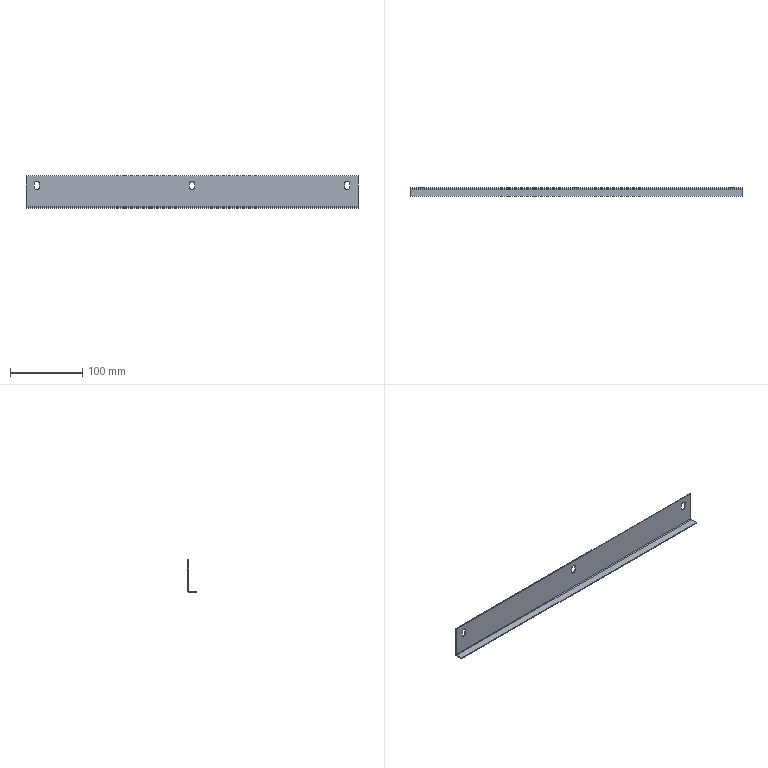Part | SolidWorks | features EdgeFlange 2, Fillet 1, FlatPattern 1, ICE 1, LPattern 1, SMBaseFlange 1, SheetMetal 1 | 1 solid | 29 faces | box 460 x 12 x 45 mm | volume 30158 mm3 | plane 18 | cylinder 11 | commonest cylinder face diameters 7 x9 2 x1 4.4 x1
STEP:
#1=CARTESIAN_POINT('',(-215.,6.,24.3));
#2=VERTEX_POINT('',#1);
#3=CARTESIAN_POINT('',(-211.5,6.,27.8));
#4=VERTEX_POINT('',#3);
#5=CARTESIAN_POINT('',(-215.,6.,27.8));
#6=DIRECTION('',(0.,-1.,0.));
#7=DIRECTION('',(0.,0.,-1.));
#8=AXIS2_PLACEMENT_3D('',#5,#6,#7);
#9=CIRCLE('',#8,3.5);
#10=EDGE_CURVE('',#2,#4,#9,.T.);
#11=ORIENTED_EDGE('',*,*,#10,.F.);
#12=CARTESIAN_POINT('',(-215.,4.8,24.3));
#13=VERTEX_POINT('',#12);
#14=CARTESIAN_POINT('',(-215.,14.8,24.3));
#15=DIRECTION('',(0.,-1.,0.));
#16=VECTOR('',#15,1000.);
#17=LINE('',#14,#16);
#18=EDGE_CURVE('',#2,#13,#17,.T.);
#19=ORIENTED_EDGE('',*,*,#18,.T.);
#20=CARTESIAN_POINT('',(-211.5,4.8,27.8));
#21=VERTEX_POINT('',#20);
#22=CARTESIAN_POINT('',(-215.,4.8,27.8));
#23=DIRECTION('',(0.,-1.,0.));
#24=DIRECTION('',(0.,0.,-1.));
#25=AXIS2_PLACEMENT_3D('',#22,#23,#24);
#26=CIRCLE('',#25,3.5);
#27=EDGE_CURVE('',#13,#21,#26,.T.);
#28=ORIENTED_EDGE('',*,*,#27,.T.);
#29=CARTESIAN_POINT('',(-211.5,14.8,27.8));
#30=DIRECTION('',(0.,-1.,0.));
#31=VECTOR('',#30,1000.);
#32=LINE('',#29,#31);
#33=EDGE_CURVE('',#4,#21,#32,.T.);
#34=ORIENTED_EDGE('',*,*,#33,.F.);
#35=EDGE_LOOP('',(#11,#19,#28,#34));
#36=FACE_OUTER_BOUND('',#35,.T.);
#37=CARTESIAN_POINT('',(-215.,14.8,27.8));
#38=DIRECTION('',(0.,-1.,0.));
#39=DIRECTION('',(0.,0.,-1.));
#40=AXIS2_PLACEMENT_3D('',#37,#38,#39);
#41=CYLINDRICAL_SURFACE('',#40,3.5);
#42=ADVANCED_FACE('',(#36),#41,.F.);
#43=CARTESIAN_POINT('',(0.,6.,24.3));
#44=VERTEX_POINT('',#43);
#45=CARTESIAN_POINT('',(3.5,6.,27.8));
#46=VERTEX_POINT('',#45);
#47=CARTESIAN_POINT('',(0.,6.,27.8));
#48=DIRECTION('',(0.,-1.,0.));
#49=DIRECTION('',(0.,0.,-1.));
#50=AXIS2_PLACEMENT_3D('',#47,#48,#49);
#51=CIRCLE('',#50,3.5);
#52=EDGE_CURVE('',#44,#46,#51,.T.);
#53=ORIENTED_EDGE('',*,*,#52,.F.);
#54=CARTESIAN_POINT('',(0.,4.8,24.3));
#55=VERTEX_POINT('',#54);
#56=CARTESIAN_POINT('',(0.,14.8,24.3));
#57=DIRECTION('',(0.,-1.,0.));
#58=VECTOR('',#57,1000.);
#59=LINE('',#56,#58);
#60=EDGE_CURVE('',#44,#55,#59,.T.);
#61=ORIENTED_EDGE('',*,*,#60,.T.);
#62=CARTESIAN_POINT('',(3.5,4.8,27.8));
#63=VERTEX_POINT('',#62);
#64=CARTESIAN_POINT('',(0.,4.8,27.8));
#65=DIRECTION('',(0.,-1.,0.));
#66=DIRECTION('',(0.,0.,-1.));
#67=AXIS2_PLACEMENT_3D('',#64,#65,#66);
#68=CIRCLE('',#67,3.5);
#69=EDGE_CURVE('',#55,#63,#68,.T.);
#70=ORIENTED_EDGE('',*,*,#69,.T.);
#71=CARTESIAN_POINT('',(3.5,14.8,27.8));
#72=DIRECTION('',(0.,-1.,0.));
#73=VECTOR('',#72,1000.);
#74=LINE('',#71,#73);
#75=EDGE_CURVE('',#46,#63,#74,.T.);
#76=ORIENTED_EDGE('',*,*,#75,.F.);
#77=EDGE_LOOP('',(#53,#61,#70,#76));
#78=FACE_OUTER_BOUND('',#77,.T.);
#79=CARTESIAN_POINT('',(0.,14.8,27.8));
#80=DIRECTION('',(0.,-1.,0.));
#81=DIRECTION('',(0.,0.,-1.));
#82=AXIS2_PLACEMENT_3D('',#79,#80,#81);
#83=CYLINDRICAL_SURFACE('',#82,3.5);
#84=ADVANCED_FACE('',(#78),#83,.F.);
#85=CARTESIAN_POINT('',(215.,6.,24.3));
#86=VERTEX_POINT('',#85);
#87=CARTESIAN_POINT('',(218.5,6.,27.8));
#88=VERTEX_POINT('',#87);
#89=CARTESIAN_POINT('',(215.,6.,27.8));
#90=DIRECTION('',(0.,-1.,0.));
#91=DIRECTION('',(0.,0.,-1.));
#92=AXIS2_PLACEMENT_3D('',#89,#90,#91);
#93=CIRCLE('',#92,3.5);
#94=EDGE_CURVE('',#86,#88,#93,.T.);
#95=ORIENTED_EDGE('',*,*,#94,.F.);
#96=CARTESIAN_POINT('',(215.,4.8,24.3));
#97=VERTEX_POINT('',#96);
#98=CARTESIAN_POINT('',(215.,14.8,24.3));
#99=DIRECTION('',(0.,-1.,0.));
#100=VECTOR('',#99,1000.);
#101=LINE('',#98,#100);
#102=EDGE_CURVE('',#86,#97,#101,.T.);
#103=ORIENTED_EDGE('',*,*,#102,.T.);
#104=CARTESIAN_POINT('',(218.5,4.8,27.8));
#105=VERTEX_POINT('',#104);
#106=CARTESIAN_POINT('',(215.,4.8,27.8));
#107=DIRECTION('',(0.,-1.,0.));
#108=DIRECTION('',(0.,0.,-1.));
#109=AXIS2_PLACEMENT_3D('',#106,#107,#108);
#110=CIRCLE('',#109,3.5);
#111=EDGE_CURVE('',#97,#105,#110,.T.);
#112=ORIENTED_EDGE('',*,*,#111,.T.);
#113=CARTESIAN_POINT('',(218.5,14.8,27.8));
#114=DIRECTION('',(0.,-1.,0.));
#115=VECTOR('',#114,1000.);
#116=LINE('',#113,#115);
#117=EDGE_CURVE('',#88,#105,#116,.T.);
#118=ORIENTED_EDGE('',*,*,#117,.F.);
#119=EDGE_LOOP('',(#95,#103,#112,#118));
#120=FACE_OUTER_BOUND('',#119,.T.);
#121=CARTESIAN_POINT('',(215.,14.8,27.8));
#122=DIRECTION('',(0.,-1.,0.));
#123=DIRECTION('',(0.,0.,-1.));
#124=AXIS2_PLACEMENT_3D('',#121,#122,#123);
#125=CYLINDRICAL_SURFACE('',#124,3.5);
#126=ADVANCED_FACE('',(#120),#125,.F.);
#127=CARTESIAN_POINT('',(218.5,6.,32.8));
#128=VERTEX_POINT('',#127);
#129=CARTESIAN_POINT('',(218.5,4.8,32.8));
#130=VERTEX_POINT('',#129);
#131=CARTESIAN_POINT('',(218.5,14.8,32.8));
#132=DIRECTION('',(0.,-1.,0.));
#133=VECTOR('',#132,1000.);
#134=LINE('',#131,#133);
#135=EDGE_CURVE('',#128,#130,#134,.T.);
#136=ORIENTED_EDGE('',*,*,#135,.T.);
#137=CARTESIAN_POINT('',(211.5,4.8,32.8));
#138=VERTEX_POINT('',#137);
#139=CARTESIAN_POINT('',(215.,4.8,32.8));
#140=DIRECTION('',(0.,-1.,0.));
#141=DIRECTION('',(0.,0.,-1.));
#142=AXIS2_PLACEMENT_3D('',#139,#140,#141);
#143=CIRCLE('',#142,3.5);
#144=EDGE_CURVE('',#130,#138,#143,.T.);
#145=ORIENTED_EDGE('',*,*,#144,.T.);
#146=CARTESIAN_POINT('',(211.5,6.,32.8));
#147=VERTEX_POINT('',#146);
#148=CARTESIAN_POINT('',(211.5,14.8,32.8));
#149=DIRECTION('',(0.,-1.,0.));
#150=VECTOR('',#149,1000.);
#151=LINE('',#148,#150);
#152=EDGE_CURVE('',#147,#138,#151,.T.);
#153=ORIENTED_EDGE('',*,*,#152,.F.);
#154=CARTESIAN_POINT('',(215.,6.,32.8));
#155=DIRECTION('',(0.,-1.,0.));
#156=DIRECTION('',(0.,0.,-1.));
#157=AXIS2_PLACEMENT_3D('',#154,#155,#156);
#158=CIRCLE('',#157,3.5);
#159=EDGE_CURVE('',#128,#147,#158,.T.);
#160=ORIENTED_EDGE('',*,*,#159,.F.);
#161=EDGE_LOOP('',(#136,#145,#153,#160));
#162=FACE_OUTER_BOUND('',#161,.T.);
#163=CARTESIAN_POINT('',(215.,14.8,32.8));
#164=DIRECTION('',(0.,-1.,0.));
#165=DIRECTION('',(0.,0.,-1.));
#166=AXIS2_PLACEMENT_3D('',#163,#164,#165);
#167=CYLINDRICAL_SURFACE('',#166,3.5);
#168=ADVANCED_FACE('',(#162),#167,.F.);
#169=ORIENTED_EDGE('',*,*,#117,.T.);
#170=CARTESIAN_POINT('',(218.5,4.8,32.8));
#171=DIRECTION('',(0.,0.,1.));
#172=VECTOR('',#171,1000.);
#173=LINE('',#170,#172);
#174=EDGE_CURVE('',#105,#130,#173,.T.);
#175=ORIENTED_EDGE('',*,*,#174,.T.);
#176=ORIENTED_EDGE('',*,*,#135,.F.);
#177=CARTESIAN_POINT('',(218.5,6.,0.));
#178=DIRECTION('',(0.,0.,1.));
#179=VECTOR('',#178,1000.);
#180=LINE('',#177,#179);
#181=EDGE_CURVE('',#88,#128,#180,.T.);
#182=ORIENTED_EDGE('',*,*,#181,.F.);
#183=EDGE_LOOP('',(#169,#175,#176,#182));
#184=FACE_OUTER_BOUND('',#183,.T.);
#185=CARTESIAN_POINT('',(218.5,14.8,32.8));
#186=DIRECTION('',(1.,0.,0.));
#187=DIRECTION('',(0.,0.,-1.));
#188=AXIS2_PLACEMENT_3D('',#185,#186,#187);
#189=PLANE('',#188);
#190=ADVANCED_FACE('',(#184),#189,.F.);
#191=ORIENTED_EDGE('',*,*,#102,.F.);
#192=CARTESIAN_POINT('',(211.5,6.,27.8));
#193=VERTEX_POINT('',#192);
#194=CARTESIAN_POINT('',(215.,6.,27.8));
#195=DIRECTION('',(0.,-1.,0.));
#196=DIRECTION('',(0.,0.,-1.));
#197=AXIS2_PLACEMENT_3D('',#194,#195,#196);
#198=CIRCLE('',#197,3.5);
#199=EDGE_CURVE('',#193,#86,#198,.T.);
#200=ORIENTED_EDGE('',*,*,#199,.F.);
#201=CARTESIAN_POINT('',(211.5,4.8,27.8));
#202=VERTEX_POINT('',#201);
#203=CARTESIAN_POINT('',(211.5,14.8,27.8));
#204=DIRECTION('',(0.,-1.,0.));
#205=VECTOR('',#204,1000.);
#206=LINE('',#203,#205);
#207=EDGE_CURVE('',#193,#202,#206,.T.);
#208=ORIENTED_EDGE('',*,*,#207,.T.);
#209=CARTESIAN_POINT('',(215.,4.8,27.8));
#210=DIRECTION('',(0.,-1.,0.));
#211=DIRECTION('',(0.,0.,-1.));
#212=AXIS2_PLACEMENT_3D('',#209,#210,#211);
#213=CIRCLE('',#212,3.5);
#214=EDGE_CURVE('',#202,#97,#213,.T.);
#215=ORIENTED_EDGE('',*,*,#214,.T.);
#216=EDGE_LOOP('',(#191,#200,#208,#215));
#217=FACE_OUTER_BOUND('',#216,.T.);
#218=CARTESIAN_POINT('',(215.,14.8,27.8));
#219=DIRECTION('',(0.,-1.,0.));
#220=DIRECTION('',(0.,0.,-1.));
#221=AXIS2_PLACEMENT_3D('',#218,#219,#220);
#222=CYLINDRICAL_SURFACE('',#221,3.5);
#223=ADVANCED_FACE('',(#217),#222,.F.);
#224=ORIENTED_EDGE('',*,*,#152,.T.);
#225=CARTESIAN_POINT('',(211.5,4.8,32.8));
#226=DIRECTION('',(0.,0.,-1.));
#227=VECTOR('',#226,1000.);
#228=LINE('',#225,#227);
#229=EDGE_CURVE('',#138,#202,#228,.T.);
#230=ORIENTED_EDGE('',*,*,#229,.T.);
#231=ORIENTED_EDGE('',*,*,#207,.F.);
#232=CARTESIAN_POINT('',(211.5,6.,0.));
#233=DIRECTION('',(0.,0.,-1.));
#234=VECTOR('',#233,1000.);
#235=LINE('',#232,#234);
#236=EDGE_CURVE('',#147,#193,#235,.T.);
#237=ORIENTED_EDGE('',*,*,#236,.F.);
#238=EDGE_LOOP('',(#224,#230,#231,#237));
#239=FACE_OUTER_BOUND('',#238,.T.);
#240=CARTESIAN_POINT('',(211.5,14.8,32.8));
#241=DIRECTION('',(-1.,0.,0.));
#242=DIRECTION('',(0.,0.,1.));
#243=AXIS2_PLACEMENT_3D('',#240,#241,#242);
#244=PLANE('',#243);
#245=ADVANCED_FACE('',(#239),#244,.F.);
#246=CARTESIAN_POINT('',(3.5,6.,32.8));
#247=VERTEX_POINT('',#246);
#248=CARTESIAN_POINT('',(3.5,4.8,32.8));
#249=VERTEX_POINT('',#248);
#250=CARTESIAN_POINT('',(3.5,14.8,32.8));
#251=DIRECTION('',(0.,-1.,0.));
#252=VECTOR('',#251,1000.);
#253=LINE('',#250,#252);
#254=EDGE_CURVE('',#247,#249,#253,.T.);
#255=ORIENTED_EDGE('',*,*,#254,.T.);
#256=CARTESIAN_POINT('',(-3.5,4.8,32.8));
#257=VERTEX_POINT('',#256);
#258=CARTESIAN_POINT('',(0.,4.8,32.8));
#259=DIRECTION('',(0.,-1.,0.));
#260=DIRECTION('',(0.,0.,-1.));
#261=AXIS2_PLACEMENT_3D('',#258,#259,#260);
#262=CIRCLE('',#261,3.5);
#263=EDGE_CURVE('',#249,#257,#262,.T.);
#264=ORIENTED_EDGE('',*,*,#263,.T.);
#265=CARTESIAN_POINT('',(-3.5,6.,32.8));
#266=VERTEX_POINT('',#265);
#267=CARTESIAN_POINT('',(-3.5,14.8,32.8));
#268=DIRECTION('',(0.,-1.,0.));
#269=VECTOR('',#268,1000.);
#270=LINE('',#267,#269);
#271=EDGE_CURVE('',#266,#257,#270,.T.);
#272=ORIENTED_EDGE('',*,*,#271,.F.);
#273=CARTESIAN_POINT('',(0.,6.,32.8));
#274=DIRECTION('',(0.,-1.,0.));
#275=DIRECTION('',(0.,0.,-1.));
#276=AXIS2_PLACEMENT_3D('',#273,#274,#275);
#277=CIRCLE('',#276,3.5);
#278=EDGE_CURVE('',#247,#266,#277,.T.);
#279=ORIENTED_EDGE('',*,*,#278,.F.);
#280=EDGE_LOOP('',(#255,#264,#272,#279));
#281=FACE_OUTER_BOUND('',#280,.T.);
#282=CARTESIAN_POINT('',(0.,14.8,32.8));
#283=DIRECTION('',(0.,-1.,0.));
#284=DIRECTION('',(0.,0.,-1.));
#285=AXIS2_PLACEMENT_3D('',#282,#283,#284);
#286=CYLINDRICAL_SURFACE('',#285,3.5);
#287=ADVANCED_FACE('',(#281),#286,.F.);
#288=ORIENTED_EDGE('',*,*,#75,.T.);
#289=CARTESIAN_POINT('',(3.5,4.8,32.8));
#290=DIRECTION('',(0.,0.,1.));
#291=VECTOR('',#290,1000.);
#292=LINE('',#289,#291);
#293=EDGE_CURVE('',#63,#249,#292,.T.);
#294=ORIENTED_EDGE('',*,*,#293,.T.);
#295=ORIENTED_EDGE('',*,*,#254,.F.);
#296=CARTESIAN_POINT('',(3.5,6.,0.));
#297=DIRECTION('',(0.,0.,1.));
#298=VECTOR('',#297,1000.);
#299=LINE('',#296,#298);
#300=EDGE_CURVE('',#46,#247,#299,.T.);
#301=ORIENTED_EDGE('',*,*,#300,.F.);
#302=EDGE_LOOP('',(#288,#294,#295,#301));
#303=FACE_OUTER_BOUND('',#302,.T.);
#304=CARTESIAN_POINT('',(3.5,14.8,32.8));
#305=DIRECTION('',(1.,0.,0.));
#306=DIRECTION('',(0.,0.,-1.));
#307=AXIS2_PLACEMENT_3D('',#304,#305,#306);
#308=PLANE('',#307);
#309=ADVANCED_FACE('',(#303),#308,.F.);
#310=ORIENTED_EDGE('',*,*,#60,.F.);
#311=CARTESIAN_POINT('',(-3.5,6.,27.8));
#312=VERTEX_POINT('',#311);
#313=CARTESIAN_POINT('',(0.,6.,27.8));
#314=DIRECTION('',(0.,-1.,0.));
#315=DIRECTION('',(0.,0.,-1.));
#316=AXIS2_PLACEMENT_3D('',#313,#314,#315);
#317=CIRCLE('',#316,3.5);
#318=EDGE_CURVE('',#312,#44,#317,.T.);
#319=ORIENTED_EDGE('',*,*,#318,.F.);
#320=CARTESIAN_POINT('',(-3.5,4.8,27.8));
#321=VERTEX_POINT('',#320);
#322=CARTESIAN_POINT('',(-3.5,14.8,27.8));
#323=DIRECTION('',(0.,-1.,0.));
#324=VECTOR('',#323,1000.);
#325=LINE('',#322,#324);
#326=EDGE_CURVE('',#312,#321,#325,.T.);
#327=ORIENTED_EDGE('',*,*,#326,.T.);
#328=CARTESIAN_POINT('',(0.,4.8,27.8));
#329=DIRECTION('',(0.,-1.,0.));
#330=DIRECTION('',(0.,0.,-1.));
#331=AXIS2_PLACEMENT_3D('',#328,#329,#330);
#332=CIRCLE('',#331,3.5);
#333=EDGE_CURVE('',#321,#55,#332,.T.);
#334=ORIENTED_EDGE('',*,*,#333,.T.);
#335=EDGE_LOOP('',(#310,#319,#327,#334));
#336=FACE_OUTER_BOUND('',#335,.T.);
#337=CARTESIAN_POINT('',(0.,14.8,27.8));
#338=DIRECTION('',(0.,-1.,0.));
#339=DIRECTION('',(0.,0.,-1.));
#340=AXIS2_PLACEMENT_3D('',#337,#338,#339);
#341=CYLINDRICAL_SURFACE('',#340,3.5);
#342=ADVANCED_FACE('',(#336),#341,.F.);
#343=ORIENTED_EDGE('',*,*,#271,.T.);
#344=CARTESIAN_POINT('',(-3.5,4.8,32.8));
#345=DIRECTION('',(0.,0.,-1.));
#346=VECTOR('',#345,1000.);
#347=LINE('',#344,#346);
#348=EDGE_CURVE('',#257,#321,#347,.T.);
#349=ORIENTED_EDGE('',*,*,#348,.T.);
#350=ORIENTED_EDGE('',*,*,#326,.F.);
#351=CARTESIAN_POINT('',(-3.5,6.,0.));
#352=DIRECTION('',(0.,0.,-1.));
#353=VECTOR('',#352,1000.);
#354=LINE('',#351,#353);
#355=EDGE_CURVE('',#266,#312,#354,.T.);
#356=ORIENTED_EDGE('',*,*,#355,.F.);
#357=EDGE_LOOP('',(#343,#349,#350,#356));
#358=FACE_OUTER_BOUND('',#357,.T.);
#359=CARTESIAN_POINT('',(-3.5,14.8,32.8));
#360=DIRECTION('',(-1.,0.,0.));
#361=DIRECTION('',(0.,0.,1.));
#362=AXIS2_PLACEMENT_3D('',#359,#360,#361);
#363=PLANE('',#362);
#364=ADVANCED_FACE('',(#358),#363,.F.);
#365=CARTESIAN_POINT('',(-230.,3.8,0.));
#366=VERTEX_POINT('',#365);
#367=CARTESIAN_POINT('',(-230.,-6.,0.));
#368=VERTEX_POINT('',#367);
#369=CARTESIAN_POINT('',(-230.,-6.,0.));
#370=DIRECTION('',(0.,-1.,0.));
#371=VECTOR('',#370,1000.);
#372=LINE('',#369,#371);
#373=EDGE_CURVE('',#366,#368,#372,.T.);
#374=ORIENTED_EDGE('',*,*,#373,.F.);
#375=CARTESIAN_POINT('',(-230.,3.8,-1.2));
#376=VERTEX_POINT('',#375);
#377=CARTESIAN_POINT('',(-230.,3.8,0.));
#378=DIRECTION('',(0.,0.,-1.));
#379=VECTOR('',#378,1000.);
#380=LINE('',#377,#379);
#381=EDGE_CURVE('',#366,#376,#380,.T.);
#382=ORIENTED_EDGE('',*,*,#381,.T.);
#383=CARTESIAN_POINT('',(-230.,-6.,-1.2));
#384=VERTEX_POINT('',#383);
#385=CARTESIAN_POINT('',(-230.,-6.,-1.2));
#386=DIRECTION('',(0.,-1.,0.));
#387=VECTOR('',#386,1000.);
#388=LINE('',#385,#387);
#389=EDGE_CURVE('',#376,#384,#388,.T.);
#390=ORIENTED_EDGE('',*,*,#389,.T.);
#391=CARTESIAN_POINT('',(-230.,-6.,-1.2));
#392=DIRECTION('',(0.,0.,1.));
#393=VECTOR('',#392,1000.);
#394=LINE('',#391,#393);
#395=EDGE_CURVE('',#384,#368,#394,.T.);
#396=ORIENTED_EDGE('',*,*,#395,.T.);
#397=EDGE_LOOP('',(#374,#382,#390,#396));
#398=FACE_OUTER_BOUND('',#397,.T.);
#399=CARTESIAN_POINT('',(-230.,-6.,-1.2));
#400=DIRECTION('',(-1.,0.,0.));
#401=DIRECTION('',(0.,0.,1.));
#402=AXIS2_PLACEMENT_3D('',#399,#400,#401);
#403=PLANE('',#402);
#404=ADVANCED_FACE('',(#398),#403,.T.);
#405=ORIENTED_EDGE('',*,*,#389,.F.);
#406=CARTESIAN_POINT('',(230.,3.8,-1.2));
#407=VERTEX_POINT('',#406);
#408=CARTESIAN_POINT('',(-230.,3.8,-1.2));
#409=DIRECTION('',(1.,0.,0.));
#410=VECTOR('',#409,1000.);
#411=LINE('',#408,#410);
#412=EDGE_CURVE('',#376,#407,#411,.T.);
#413=ORIENTED_EDGE('',*,*,#412,.T.);
#414=CARTESIAN_POINT('',(230.,-6.,-1.2));
#415=VERTEX_POINT('',#414);
#416=CARTESIAN_POINT('',(230.,-6.,-1.2));
#417=DIRECTION('',(0.,1.,0.));
#418=VECTOR('',#417,1000.);
#419=LINE('',#416,#418);
#420=EDGE_CURVE('',#415,#407,#419,.T.);
#421=ORIENTED_EDGE('',*,*,#420,.F.);
#422=CARTESIAN_POINT('',(-230.,-6.,-1.2));
#423=DIRECTION('',(1.,0.,0.));
#424=VECTOR('',#423,1000.);
#425=LINE('',#422,#424);
#426=EDGE_CURVE('',#384,#415,#425,.T.);
#427=ORIENTED_EDGE('',*,*,#426,.F.);
#428=EDGE_LOOP('',(#405,#413,#421,#427));
#429=FACE_OUTER_BOUND('',#428,.T.);
#430=CARTESIAN_POINT('',(0.,0.,-1.2));
#431=DIRECTION('',(0.,0.,-1.));
#432=DIRECTION('',(-1.,0.,0.));
#433=AXIS2_PLACEMENT_3D('',#430,#431,#432);
#434=PLANE('',#433);
#435=ADVANCED_FACE('',(#429),#434,.T.);
#436=CARTESIAN_POINT('',(230.,3.8,0.));
#437=VERTEX_POINT('',#436);
#438=CARTESIAN_POINT('',(-230.,3.8,0.));
#439=DIRECTION('',(1.,0.,0.));
#440=VECTOR('',#439,1000.);
#441=LINE('',#438,#440);
#442=EDGE_CURVE('',#366,#437,#441,.T.);
#443=ORIENTED_EDGE('',*,*,#442,.F.);
#444=ORIENTED_EDGE('',*,*,#373,.T.);
#445=CARTESIAN_POINT('',(230.,-6.,0.));
#446=VERTEX_POINT('',#445);
#447=CARTESIAN_POINT('',(-230.,-6.,0.));
#448=DIRECTION('',(1.,0.,0.));
#449=VECTOR('',#448,1000.);
#450=LINE('',#447,#449);
#451=EDGE_CURVE('',#368,#446,#450,.T.);
#452=ORIENTED_EDGE('',*,*,#451,.T.);
#453=CARTESIAN_POINT('',(230.,-6.,0.));
#454=DIRECTION('',(0.,1.,0.));
#455=VECTOR('',#454,1000.);
#456=LINE('',#453,#455);
#457=EDGE_CURVE('',#446,#437,#456,.T.);
#458=ORIENTED_EDGE('',*,*,#457,.T.);
#459=EDGE_LOOP('',(#443,#444,#452,#458));
#460=FACE_OUTER_BOUND('',#459,.T.);
#461=CARTESIAN_POINT('',(0.,0.,0.));
#462=DIRECTION('',(0.,0.,-1.));
#463=DIRECTION('',(-1.,0.,0.));
#464=AXIS2_PLACEMENT_3D('',#461,#462,#463);
#465=PLANE('',#464);
#466=ADVANCED_FACE('',(#460),#465,.F.);
#467=CARTESIAN_POINT('',(230.,3.8,0.));
#468=DIRECTION('',(0.,0.,-1.));
#469=VECTOR('',#468,1000.);
#470=LINE('',#467,#469);
#471=EDGE_CURVE('',#437,#407,#470,.T.);
#472=ORIENTED_EDGE('',*,*,#471,.F.);
#473=ORIENTED_EDGE('',*,*,#457,.F.);
#474=CARTESIAN_POINT('',(230.,-6.,-1.2));
#475=DIRECTION('',(0.,0.,1.));
#476=VECTOR('',#475,1000.);
#477=LINE('',#474,#476);
#478=EDGE_CURVE('',#415,#446,#477,.T.);
#479=ORIENTED_EDGE('',*,*,#478,.F.);
#480=ORIENTED_EDGE('',*,*,#420,.T.);
#481=EDGE_LOOP('',(#472,#473,#479,#480));
#482=FACE_OUTER_BOUND('',#481,.T.);
#483=CARTESIAN_POINT('',(230.,-6.,-1.2));
#484=DIRECTION('',(1.,0.,0.));
#485=DIRECTION('',(0.,0.,-1.));
#486=AXIS2_PLACEMENT_3D('',#483,#484,#485);
#487=PLANE('',#486);
#488=ADVANCED_FACE('',(#482),#487,.T.);
#489=ORIENTED_EDGE('',*,*,#451,.F.);
#490=ORIENTED_EDGE('',*,*,#395,.F.);
#491=ORIENTED_EDGE('',*,*,#426,.T.);
#492=ORIENTED_EDGE('',*,*,#478,.T.);
#493=EDGE_LOOP('',(#489,#490,#491,#492));
#494=FACE_OUTER_BOUND('',#493,.T.);
#495=CARTESIAN_POINT('',(-230.,-6.,-1.2));
#496=DIRECTION('',(0.,-1.,0.));
#497=DIRECTION('',(0.,0.,-1.));
#498=AXIS2_PLACEMENT_3D('',#495,#496,#497);
#499=PLANE('',#498);
#500=ADVANCED_FACE('',(#494),#499,.T.);
#501=CARTESIAN_POINT('',(230.,4.8,1.));
#502=VERTEX_POINT('',#501);
#503=CARTESIAN_POINT('',(230.,6.,1.));
#504=VERTEX_POINT('',#503);
#505=CARTESIAN_POINT('',(230.,6.,1.));
#506=DIRECTION('',(0.,1.,0.));
#507=VECTOR('',#506,1000.);
#508=LINE('',#505,#507);
#509=EDGE_CURVE('',#502,#504,#508,.T.);
#510=ORIENTED_EDGE('',*,*,#509,.F.);
#511=CARTESIAN_POINT('',(230.,3.8,1.));
#512=DIRECTION('',(1.,0.,0.));
#513=DIRECTION('',(0.,0.,1.));
#514=AXIS2_PLACEMENT_3D('',#511,#512,#513);
#515=CIRCLE('',#514,1.);
#516=EDGE_CURVE('',#437,#502,#515,.T.);
#517=ORIENTED_EDGE('',*,*,#516,.F.);
#518=ORIENTED_EDGE('',*,*,#471,.T.);
#519=CARTESIAN_POINT('',(230.,3.8,1.));
#520=DIRECTION('',(1.,0.,0.));
#521=DIRECTION('',(0.,0.,1.));
#522=AXIS2_PLACEMENT_3D('',#519,#520,#521);
#523=CIRCLE('',#522,2.2);
#524=EDGE_CURVE('',#407,#504,#523,.T.);
#525=ORIENTED_EDGE('',*,*,#524,.T.);
#526=EDGE_LOOP('',(#510,#517,#518,#525));
#527=FACE_OUTER_BOUND('',#526,.T.);
#528=CARTESIAN_POINT('',(230.,3.8,1.));
#529=DIRECTION('',(1.,0.,0.));
#530=DIRECTION('',(0.,0.,-1.));
#531=AXIS2_PLACEMENT_3D('',#528,#529,#530);
#532=PLANE('',#531);
#533=ADVANCED_FACE('',(#527),#532,.T.);
#534=CARTESIAN_POINT('',(-230.,4.8,1.));
#535=VERTEX_POINT('',#534);
#536=CARTESIAN_POINT('',(-230.,3.8,1.));
#537=DIRECTION('',(-1.,0.,0.));
#538=DIRECTION('',(0.,0.,1.));
#539=AXIS2_PLACEMENT_3D('',#536,#537,#538);
#540=CIRCLE('',#539,1.);
#541=EDGE_CURVE('',#535,#366,#540,.T.);
#542=ORIENTED_EDGE('',*,*,#541,.F.);
#543=CARTESIAN_POINT('',(-230.,6.,1.));
#544=VERTEX_POINT('',#543);
#545=CARTESIAN_POINT('',(-230.,4.8,1.));
#546=DIRECTION('',(0.,1.,0.));
#547=VECTOR('',#546,1000.);
#548=LINE('',#545,#547);
#549=EDGE_CURVE('',#535,#544,#548,.T.);
#550=ORIENTED_EDGE('',*,*,#549,.T.);
#551=CARTESIAN_POINT('',(-230.,3.8,1.));
#552=DIRECTION('',(-1.,0.,0.));
#553=DIRECTION('',(0.,0.,1.));
#554=AXIS2_PLACEMENT_3D('',#551,#552,#553);
#555=CIRCLE('',#554,2.2);
#556=EDGE_CURVE('',#544,#376,#555,.T.);
#557=ORIENTED_EDGE('',*,*,#556,.T.);
#558=ORIENTED_EDGE('',*,*,#381,.F.);
#559=EDGE_LOOP('',(#542,#550,#557,#558));
#560=FACE_OUTER_BOUND('',#559,.T.);
#561=CARTESIAN_POINT('',(-230.,3.8,1.));
#562=DIRECTION('',(1.,0.,0.));
#563=DIRECTION('',(0.,0.,-1.));
#564=AXIS2_PLACEMENT_3D('',#561,#562,#563);
#565=PLANE('',#564);
#566=ADVANCED_FACE('',(#560),#565,.F.);
#567=ORIENTED_EDGE('',*,*,#412,.F.);
#568=ORIENTED_EDGE('',*,*,#556,.F.);
#569=CARTESIAN_POINT('',(230.,6.,1.));
#570=DIRECTION('',(1.,0.,0.));
#571=VECTOR('',#570,1000.);
#572=LINE('',#569,#571);
#573=EDGE_CURVE('',#544,#504,#572,.T.);
#574=ORIENTED_EDGE('',*,*,#573,.T.);
#575=ORIENTED_EDGE('',*,*,#524,.F.);
#576=EDGE_LOOP('',(#567,#568,#574,#575));
#577=FACE_OUTER_BOUND('',#576,.T.);
#578=CARTESIAN_POINT('',(-230.,3.8,1.));
#579=DIRECTION('',(-1.,0.,0.));
#580=DIRECTION('',(0.,1.,0.));
#581=AXIS2_PLACEMENT_3D('',#578,#579,#580);
#582=CYLINDRICAL_SURFACE('',#581,2.2);
#583=ADVANCED_FACE('',(#577),#582,.T.);
#584=ORIENTED_EDGE('',*,*,#442,.T.);
#585=ORIENTED_EDGE('',*,*,#516,.T.);
#586=CARTESIAN_POINT('',(230.,4.8,1.));
#587=DIRECTION('',(-1.,0.,0.));
#588=VECTOR('',#587,1000.);
#589=LINE('',#586,#588);
#590=EDGE_CURVE('',#502,#535,#589,.T.);
#591=ORIENTED_EDGE('',*,*,#590,.T.);
#592=ORIENTED_EDGE('',*,*,#541,.T.);
#593=EDGE_LOOP('',(#584,#585,#591,#592));
#594=FACE_OUTER_BOUND('',#593,.T.);
#595=CARTESIAN_POINT('',(-230.,3.8,1.));
#596=DIRECTION('',(-1.,0.,0.));
#597=DIRECTION('',(0.,1.,0.));
#598=AXIS2_PLACEMENT_3D('',#595,#596,#597);
#599=CYLINDRICAL_SURFACE('',#598,1.);
#600=ADVANCED_FACE('',(#594),#599,.F.);
#601=ORIENTED_EDGE('',*,*,#509,.T.);
#602=CARTESIAN_POINT('',(230.,6.,43.8));
#603=VERTEX_POINT('',#602);
#604=CARTESIAN_POINT('',(230.,6.,0.));
#605=DIRECTION('',(0.,0.,-1.));
#606=VECTOR('',#605,1000.);
#607=LINE('',#604,#606);
#608=EDGE_CURVE('',#603,#504,#607,.T.);
#609=ORIENTED_EDGE('',*,*,#608,.F.);
#610=CARTESIAN_POINT('',(230.,4.8,43.8));
#611=VERTEX_POINT('',#610);
#612=CARTESIAN_POINT('',(230.,6.,43.8));
#613=DIRECTION('',(0.,-1.,0.));
#614=VECTOR('',#613,1000.);
#615=LINE('',#612,#614);
#616=EDGE_CURVE('',#603,#611,#615,.T.);
#617=ORIENTED_EDGE('',*,*,#616,.T.);
#618=CARTESIAN_POINT('',(230.,4.8,0.));
#619=DIRECTION('',(0.,0.,-1.));
#620=VECTOR('',#619,1000.);
#621=LINE('',#618,#620);
#622=EDGE_CURVE('',#611,#502,#621,.T.);
#623=ORIENTED_EDGE('',*,*,#622,.T.);
#624=EDGE_LOOP('',(#601,#609,#617,#623));
#625=FACE_OUTER_BOUND('',#624,.T.);
#626=CARTESIAN_POINT('',(230.,6.,0.));
#627=DIRECTION('',(-1.,0.,0.));
#628=DIRECTION('',(0.,0.,1.));
#629=AXIS2_PLACEMENT_3D('',#626,#627,#628);
#630=PLANE('',#629);
#631=ADVANCED_FACE('',(#625),#630,.F.);
#632=ORIENTED_EDGE('',*,*,#549,.F.);
#633=CARTESIAN_POINT('',(-230.,4.8,43.8));
#634=VERTEX_POINT('',#633);
#635=CARTESIAN_POINT('',(-230.,4.8,43.8));
#636=DIRECTION('',(0.,0.,1.));
#637=VECTOR('',#636,1000.);
#638=LINE('',#635,#637);
#639=EDGE_CURVE('',#535,#634,#638,.T.);
#640=ORIENTED_EDGE('',*,*,#639,.T.);
#641=CARTESIAN_POINT('',(-230.,6.,43.8));
#642=VERTEX_POINT('',#641);
#643=CARTESIAN_POINT('',(-230.,6.,43.8));
#644=DIRECTION('',(0.,-1.,0.));
#645=VECTOR('',#644,1000.);
#646=LINE('',#643,#645);
#647=EDGE_CURVE('',#642,#634,#646,.T.);
#648=ORIENTED_EDGE('',*,*,#647,.F.);
#649=CARTESIAN_POINT('',(-230.,6.,0.));
#650=DIRECTION('',(0.,0.,1.));
#651=VECTOR('',#650,1000.);
#652=LINE('',#649,#651);
#653=EDGE_CURVE('',#544,#642,#652,.T.);
#654=ORIENTED_EDGE('',*,*,#653,.F.);
#655=EDGE_LOOP('',(#632,#640,#648,#654));
#656=FACE_OUTER_BOUND('',#655,.T.);
#657=CARTESIAN_POINT('',(-230.,6.,43.8));
#658=DIRECTION('',(1.,0.,0.));
#659=DIRECTION('',(0.,0.,-1.));
#660=AXIS2_PLACEMENT_3D('',#657,#658,#659);
#661=PLANE('',#660);
#662=ADVANCED_FACE('',(#656),#661,.F.);
#663=ORIENTED_EDGE('',*,*,#181,.T.);
#664=ORIENTED_EDGE('',*,*,#159,.T.);
#665=ORIENTED_EDGE('',*,*,#236,.T.);
#666=ORIENTED_EDGE('',*,*,#199,.T.);
#667=ORIENTED_EDGE('',*,*,#94,.T.);
#668=EDGE_LOOP('',(#663,#664,#665,#666,#667));
#669=FACE_BOUND('',#668,.T.);
#670=ORIENTED_EDGE('',*,*,#300,.T.);
#671=ORIENTED_EDGE('',*,*,#278,.T.);
#672=ORIENTED_EDGE('',*,*,#355,.T.);
#673=ORIENTED_EDGE('',*,*,#318,.T.);
#674=ORIENTED_EDGE('',*,*,#52,.T.);
#675=EDGE_LOOP('',(#670,#671,#672,#673,#674));
#676=FACE_BOUND('',#675,.T.);
#677=CARTESIAN_POINT('',(-211.5,6.,32.8));
#678=VERTEX_POINT('',#677);
#679=CARTESIAN_POINT('',(-211.5,6.,0.));
#680=DIRECTION('',(0.,0.,1.));
#681=VECTOR('',#680,1000.);
#682=LINE('',#679,#681);
#683=EDGE_CURVE('',#4,#678,#682,.T.);
#684=ORIENTED_EDGE('',*,*,#683,.T.);
#685=CARTESIAN_POINT('',(-218.5,6.,32.8));
#686=VERTEX_POINT('',#685);
#687=CARTESIAN_POINT('',(-215.,6.,32.8));
#688=DIRECTION('',(0.,-1.,0.));
#689=DIRECTION('',(0.,0.,-1.));
#690=AXIS2_PLACEMENT_3D('',#687,#688,#689);
#691=CIRCLE('',#690,3.5);
#692=EDGE_CURVE('',#678,#686,#691,.T.);
#693=ORIENTED_EDGE('',*,*,#692,.T.);
#694=CARTESIAN_POINT('',(-218.5,6.,27.8));
#695=VERTEX_POINT('',#694);
#696=CARTESIAN_POINT('',(-218.5,6.,0.));
#697=DIRECTION('',(0.,0.,-1.));
#698=VECTOR('',#697,1000.);
#699=LINE('',#696,#698);
#700=EDGE_CURVE('',#686,#695,#699,.T.);
#701=ORIENTED_EDGE('',*,*,#700,.T.);
#702=CARTESIAN_POINT('',(-215.,6.,27.8));
#703=DIRECTION('',(0.,-1.,0.));
#704=DIRECTION('',(0.,0.,-1.));
#705=AXIS2_PLACEMENT_3D('',#702,#703,#704);
#706=CIRCLE('',#705,3.5);
#707=EDGE_CURVE('',#695,#2,#706,.T.);
#708=ORIENTED_EDGE('',*,*,#707,.T.);
#709=ORIENTED_EDGE('',*,*,#10,.T.);
#710=EDGE_LOOP('',(#684,#693,#701,#708,#709));
#711=FACE_BOUND('',#710,.T.);
#712=ORIENTED_EDGE('',*,*,#573,.F.);
#713=ORIENTED_EDGE('',*,*,#653,.T.);
#714=CARTESIAN_POINT('',(0.,6.,43.8));
#715=DIRECTION('',(1.,0.,0.));
#716=VECTOR('',#715,1000.);
#717=LINE('',#714,#716);
#718=EDGE_CURVE('',#642,#603,#717,.T.);
#719=ORIENTED_EDGE('',*,*,#718,.T.);
#720=ORIENTED_EDGE('',*,*,#608,.T.);
#721=EDGE_LOOP('',(#712,#713,#719,#720));
#722=FACE_OUTER_BOUND('',#721,.T.);
#723=CARTESIAN_POINT('',(0.,6.,0.));
#724=DIRECTION('',(0.,-1.,0.));
#725=DIRECTION('',(0.,0.,-1.));
#726=AXIS2_PLACEMENT_3D('',#723,#724,#725);
#727=PLANE('',#726);
#728=ADVANCED_FACE('',(#669,#676,#711,#722),#727,.F.);
#729=ORIENTED_EDGE('',*,*,#144,.F.);
#730=ORIENTED_EDGE('',*,*,#174,.F.);
#731=ORIENTED_EDGE('',*,*,#111,.F.);
#732=ORIENTED_EDGE('',*,*,#214,.F.);
#733=ORIENTED_EDGE('',*,*,#229,.F.);
#734=EDGE_LOOP('',(#729,#730,#731,#732,#733));
#735=FACE_BOUND('',#734,.T.);
#736=ORIENTED_EDGE('',*,*,#263,.F.);
#737=ORIENTED_EDGE('',*,*,#293,.F.);
#738=ORIENTED_EDGE('',*,*,#69,.F.);
#739=ORIENTED_EDGE('',*,*,#333,.F.);
#740=ORIENTED_EDGE('',*,*,#348,.F.);
#741=EDGE_LOOP('',(#736,#737,#738,#739,#740));
#742=FACE_BOUND('',#741,.T.);
#743=CARTESIAN_POINT('',(-211.5,4.8,32.8));
#744=VERTEX_POINT('',#743);
#745=CARTESIAN_POINT('',(-218.5,4.8,32.8));
#746=VERTEX_POINT('',#745);
#747=CARTESIAN_POINT('',(-215.,4.8,32.8));
#748=DIRECTION('',(0.,-1.,0.));
#749=DIRECTION('',(0.,0.,-1.));
#750=AXIS2_PLACEMENT_3D('',#747,#748,#749);
#751=CIRCLE('',#750,3.5);
#752=EDGE_CURVE('',#744,#746,#751,.T.);
#753=ORIENTED_EDGE('',*,*,#752,.F.);
#754=CARTESIAN_POINT('',(-211.5,4.8,32.8));
#755=DIRECTION('',(0.,0.,1.));
#756=VECTOR('',#755,1000.);
#757=LINE('',#754,#756);
#758=EDGE_CURVE('',#21,#744,#757,.T.);
#759=ORIENTED_EDGE('',*,*,#758,.F.);
#760=ORIENTED_EDGE('',*,*,#27,.F.);
#761=CARTESIAN_POINT('',(-218.5,4.8,27.8));
#762=VERTEX_POINT('',#761);
#763=CARTESIAN_POINT('',(-215.,4.8,27.8));
#764=DIRECTION('',(0.,-1.,0.));
#765=DIRECTION('',(0.,0.,-1.));
#766=AXIS2_PLACEMENT_3D('',#763,#764,#765);
#767=CIRCLE('',#766,3.5);
#768=EDGE_CURVE('',#762,#13,#767,.T.);
#769=ORIENTED_EDGE('',*,*,#768,.F.);
#770=CARTESIAN_POINT('',(-218.5,4.8,32.8));
#771=DIRECTION('',(0.,0.,-1.));
#772=VECTOR('',#771,1000.);
#773=LINE('',#770,#772);
#774=EDGE_CURVE('',#746,#762,#773,.T.);
#775=ORIENTED_EDGE('',*,*,#774,.F.);
#776=EDGE_LOOP('',(#753,#759,#760,#769,#775));
#777=FACE_BOUND('',#776,.T.);
#778=ORIENTED_EDGE('',*,*,#639,.F.);
#779=ORIENTED_EDGE('',*,*,#590,.F.);
#780=ORIENTED_EDGE('',*,*,#622,.F.);
#781=CARTESIAN_POINT('',(230.,4.8,43.8));
#782=DIRECTION('',(1.,0.,0.));
#783=VECTOR('',#782,1000.);
#784=LINE('',#781,#783);
#785=EDGE_CURVE('',#634,#611,#784,.T.);
#786=ORIENTED_EDGE('',*,*,#785,.F.);
#787=EDGE_LOOP('',(#778,#779,#780,#786));
#788=FACE_OUTER_BOUND('',#787,.T.);
#789=CARTESIAN_POINT('',(0.,4.8,0.));
#790=DIRECTION('',(0.,-1.,0.));
#791=DIRECTION('',(0.,0.,-1.));
#792=AXIS2_PLACEMENT_3D('',#789,#790,#791);
#793=PLANE('',#792);
#794=ADVANCED_FACE('',(#735,#742,#777,#788),#793,.T.);
#795=ORIENTED_EDGE('',*,*,#785,.T.);
#796=ORIENTED_EDGE('',*,*,#616,.F.);
#797=ORIENTED_EDGE('',*,*,#718,.F.);
#798=ORIENTED_EDGE('',*,*,#647,.T.);
#799=EDGE_LOOP('',(#795,#796,#797,#798));
#800=FACE_OUTER_BOUND('',#799,.T.);
#801=CARTESIAN_POINT('',(230.,6.,43.8));
#802=DIRECTION('',(0.,0.,-1.));
#803=DIRECTION('',(0.,1.,0.));
#804=AXIS2_PLACEMENT_3D('',#801,#802,#803);
#805=PLANE('',#804);
#806=ADVANCED_FACE('',(#800),#805,.F.);
#807=CARTESIAN_POINT('',(-211.5,14.8,32.8));
#808=DIRECTION('',(0.,-1.,0.));
#809=VECTOR('',#808,1000.);
#810=LINE('',#807,#809);
#811=EDGE_CURVE('',#678,#744,#810,.T.);
#812=ORIENTED_EDGE('',*,*,#811,.T.);
#813=ORIENTED_EDGE('',*,*,#752,.T.);
#814=CARTESIAN_POINT('',(-218.5,14.8,32.8));
#815=DIRECTION('',(0.,-1.,0.));
#816=VECTOR('',#815,1000.);
#817=LINE('',#814,#816);
#818=EDGE_CURVE('',#686,#746,#817,.T.);
#819=ORIENTED_EDGE('',*,*,#818,.F.);
#820=ORIENTED_EDGE('',*,*,#692,.F.);
#821=EDGE_LOOP('',(#812,#813,#819,#820));
#822=FACE_OUTER_BOUND('',#821,.T.);
#823=CARTESIAN_POINT('',(-215.,14.8,32.8));
#824=DIRECTION('',(0.,-1.,0.));
#825=DIRECTION('',(0.,0.,-1.));
#826=AXIS2_PLACEMENT_3D('',#823,#824,#825);
#827=CYLINDRICAL_SURFACE('',#826,3.5);
#828=ADVANCED_FACE('',(#822),#827,.F.);
#829=ORIENTED_EDGE('',*,*,#33,.T.);
#830=ORIENTED_EDGE('',*,*,#758,.T.);
#831=ORIENTED_EDGE('',*,*,#811,.F.);
#832=ORIENTED_EDGE('',*,*,#683,.F.);
#833=EDGE_LOOP('',(#829,#830,#831,#832));
#834=FACE_OUTER_BOUND('',#833,.T.);
#835=CARTESIAN_POINT('',(-211.5,14.8,32.8));
#836=DIRECTION('',(1.,0.,0.));
#837=DIRECTION('',(0.,0.,-1.));
#838=AXIS2_PLACEMENT_3D('',#835,#836,#837);
#839=PLANE('',#838);
#840=ADVANCED_FACE('',(#834),#839,.F.);
#841=ORIENTED_EDGE('',*,*,#18,.F.);
#842=ORIENTED_EDGE('',*,*,#707,.F.);
#843=CARTESIAN_POINT('',(-218.5,14.8,27.8));
#844=DIRECTION('',(0.,-1.,0.));
#845=VECTOR('',#844,1000.);
#846=LINE('',#843,#845);
#847=EDGE_CURVE('',#695,#762,#846,.T.);
#848=ORIENTED_EDGE('',*,*,#847,.T.);
#849=ORIENTED_EDGE('',*,*,#768,.T.);
#850=EDGE_LOOP('',(#841,#842,#848,#849));
#851=FACE_OUTER_BOUND('',#850,.T.);
#852=CARTESIAN_POINT('',(-215.,14.8,27.8));
#853=DIRECTION('',(0.,-1.,0.));
#854=DIRECTION('',(0.,0.,-1.));
#855=AXIS2_PLACEMENT_3D('',#852,#853,#854);
#856=CYLINDRICAL_SURFACE('',#855,3.5);
#857=ADVANCED_FACE('',(#851),#856,.F.);
#858=ORIENTED_EDGE('',*,*,#818,.T.);
#859=ORIENTED_EDGE('',*,*,#774,.T.);
#860=ORIENTED_EDGE('',*,*,#847,.F.);
#861=ORIENTED_EDGE('',*,*,#700,.F.);
#862=EDGE_LOOP('',(#858,#859,#860,#861));
#863=FACE_OUTER_BOUND('',#862,.T.);
#864=CARTESIAN_POINT('',(-218.5,14.8,32.8));
#865=DIRECTION('',(-1.,0.,0.));
#866=DIRECTION('',(0.,0.,1.));
#867=AXIS2_PLACEMENT_3D('',#864,#865,#866);
#868=PLANE('',#867);
#869=ADVANCED_FACE('',(#863),#868,.F.);
#870=CLOSED_SHELL('',(#42,#84,#126,#168,#190,#223,#245,#287,#309,#342,#364,#404,#435,#466,#488,#500,#533,#566,#583,#600,#631,#662,#728,#794,#806,#828,#840,#857,#869));
#871=MANIFOLD_SOLID_BREP('',#870);
#872=CARTESIAN_POINT('',(0.,0.,0.));
#873=DIRECTION('',(0.,0.,1.));
#874=DIRECTION('',(1.,0.,0.));
#875=AXIS2_PLACEMENT_3D('',#872,#873,#874);
#876=(LENGTH_UNIT()NAMED_UNIT(*)SI_UNIT(.MILLI.,.METRE.));
#877=UNCERTAINTY_MEASURE_WITH_UNIT(LENGTH_MEASURE(0.00001),#876,'','');
#878=(NAMED_UNIT(*)PLANE_ANGLE_UNIT()SI_UNIT($,.RADIAN.));
#879=(NAMED_UNIT(*)SI_UNIT($,.STERADIAN.)SOLID_ANGLE_UNIT());
#880=(GEOMETRIC_REPRESENTATION_CONTEXT(3)GLOBAL_UNCERTAINTY_ASSIGNED_CONTEXT((#877))GLOBAL_UNIT_ASSIGNED_CONTEXT((#876,#878,#879))REPRESENTATION_CONTEXT('',''));
#881=ADVANCED_BREP_SHAPE_REPRESENTATION('',(#871,#875),#880);